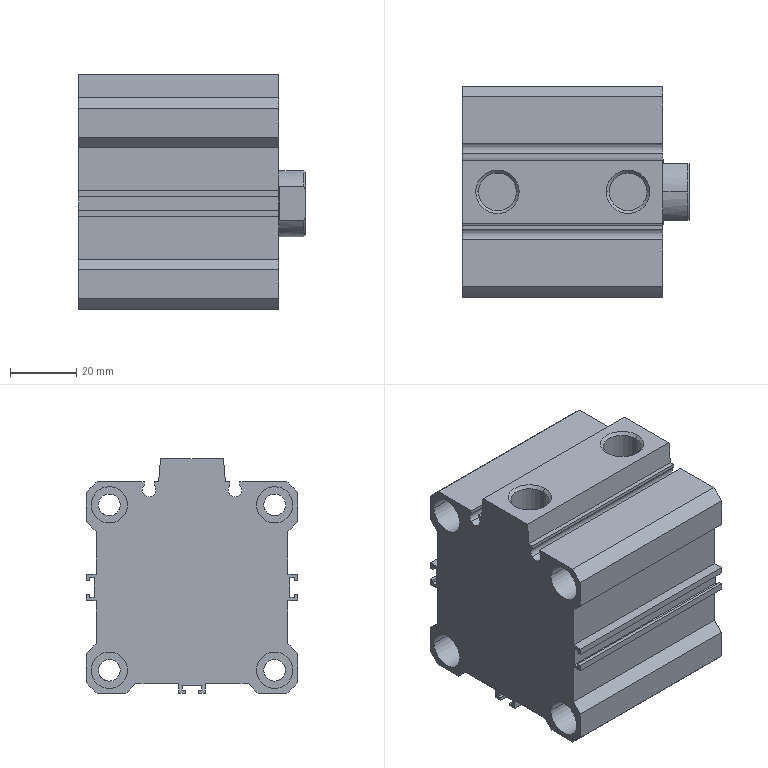Part | STEP file | Positioning_id2298_x_t | 1 solid | 131 faces | box 68.5 x 64 x 71 mm | volume 221302 mm3 | plane 79 | cylinder 40 | cone 12 | commonest cylinder face diameters 11 x16 6.6 x8 4.2 x4 11.45 x4 86 x4 8.16 x2